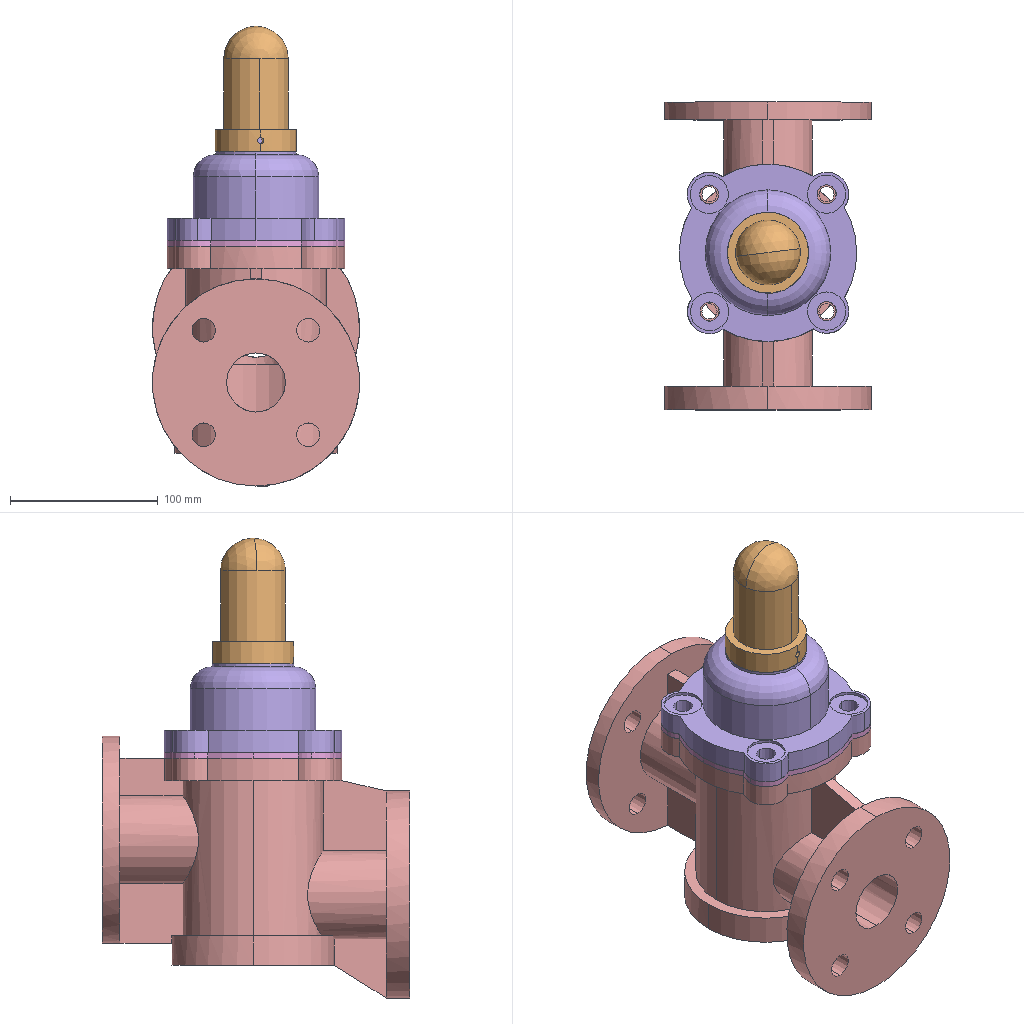Assembly | SolidWorks | 7 different items | 7 placed | box 140 x 208 x 311 mm
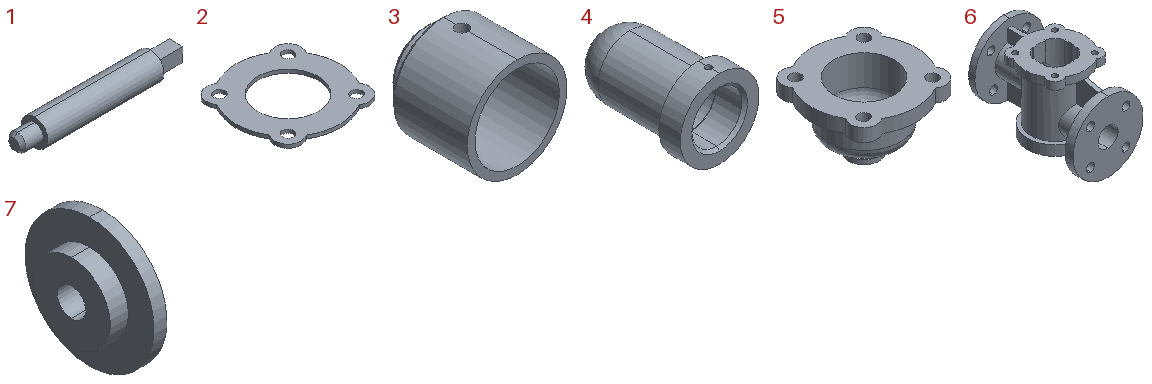Parts list (item | quantity | size | volume | features):
1 | x1 | 95 x 15.69 x 15.69 mm | 14996 mm3 | features Chamfer 1, ICE 1, Revolution 1
2 | x1 | 120 x 120 x 4 mm | 31763 mm3 | features Extrusion 1
3 | x1 | 65 x 60 x 65 mm | 87654 mm3 | features Chamfer 2, ICE 2, RevCut 2, Revolution 1
4 | x1 | 55 x 85 x 55 mm | 61984 mm3 | features 3DProfileFeature 1, Chamfer 1, HoleWzd 1, Revolution 1
5 | x1 | 120 x 120 x 75 mm | 236735 mm3 | features ICE 4, Fillet 2, Extrusion 1, Revolution 1
6 | x1 | 140 x 208 x 177 mm | 1195368 mm3 | features ICE 14, RevCut 3, 3DProfileFeature 1, Chamfer 1, CirPattern 1, CombineBodies 1, Extrusion 1, HoleWzd 1, Split 1
7 | x1 | 12 x 50 x 50 mm | 13625 mm3 | features ICE 1, Revolution 1
Mates (type | each side: item.copy, entity, surface, feature):
Concentric | 7.1 face cylinder Cut-Extrude1 | 1.1 face cylinder Revolve1
Coincident | 7.1 face plane Revolve1 | 1.1 face plane Revolve1
Concentric | 6.1 face cylinder Cut-Revolve2 | 3.1 face cylinder Revolve1
Coincident | 6.1 face cone Chamfer2 | 3.1 face cone Chamfer1
Concentric | 1.1 face cylinder Revolve1 | 5.1 face cylinder Cut-Extrude2
Concentric | 6.1 face cylinder Boss-Extrude2 | 2.1 face cylinder Boss-Extrude1 | 2 times
Coincident | 6.1 face plane Boss-Extrude1 | 2.1 face plane Boss-Extrude1
Coincident | 7.1 face plane Revolve1 | 5.1 face plane Cut-Extrude3
Concentric | 4.1 face cylinder Revolve2 | 5.1 face cylinder Revolve1
Coincident | 4.1 face plane Revolve2 | 5.1 face plane Boss-Extrude2
Concentric | 6.1 face cylinder Boss-Extrude2 | 5.1 face cylinder Boss-Extrude1
Coincident | 2.1 face plane Boss-Extrude1 | 5.1 face plane Boss-Extrude1
Concentric | 3.1 face cylinder Cut-Revolve1 | 5.1 face cylinder Cut-Extrude3